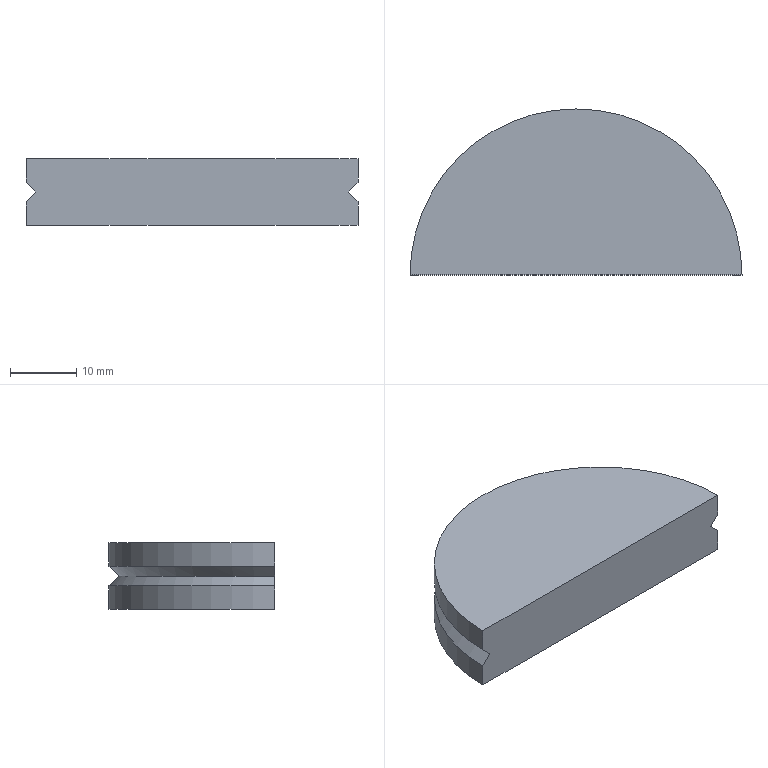Part | SolidWorks | features Extrusion 1, SweepCut 1 | 1 solid | 7 faces | box 50 x 25 x 10 mm | volume 9644 mm3 | plane 3 | cylinder 2 | cone 2 | commonest cylinder face diameters 50 x2
STEP:
#1=CARTESIAN_POINT('',(26.255,-21.468,10.));
#2=VERTEX_POINT('',#1);
#3=CARTESIAN_POINT('',(26.255,-21.468,6.5));
#4=VERTEX_POINT('',#3);
#5=CARTESIAN_POINT('',(26.255,-21.468,10.));
#6=DIRECTION('',(0.,0.,-1.));
#7=VECTOR('',#6,1000.);
#8=LINE('',#5,#7);
#9=EDGE_CURVE('',#2,#4,#8,.T.);
#10=ORIENTED_EDGE('',*,*,#9,.T.);
#11=CARTESIAN_POINT('',(-23.745,-21.468,6.5));
#12=VERTEX_POINT('',#11);
#13=CARTESIAN_POINT('',(1.255,-21.468,6.5));
#14=DIRECTION('',(0.,0.,-1.));
#15=DIRECTION('',(-1.,0.,0.));
#16=AXIS2_PLACEMENT_3D('',#13,#14,#15);
#17=CIRCLE('',#16,25.);
#18=EDGE_CURVE('',#12,#4,#17,.T.);
#19=ORIENTED_EDGE('',*,*,#18,.F.);
#20=CARTESIAN_POINT('',(-23.745,-21.468,10.));
#21=VERTEX_POINT('',#20);
#22=CARTESIAN_POINT('',(-23.745,-21.468,10.));
#23=DIRECTION('',(0.,0.,-1.));
#24=VECTOR('',#23,1000.);
#25=LINE('',#22,#24);
#26=EDGE_CURVE('',#21,#12,#25,.T.);
#27=ORIENTED_EDGE('',*,*,#26,.F.);
#28=CARTESIAN_POINT('',(1.255,-21.468,10.));
#29=DIRECTION('',(0.,0.,1.));
#30=DIRECTION('',(1.,0.,0.));
#31=AXIS2_PLACEMENT_3D('',#28,#29,#30);
#32=CIRCLE('',#31,25.);
#33=EDGE_CURVE('',#2,#21,#32,.T.);
#34=ORIENTED_EDGE('',*,*,#33,.F.);
#35=EDGE_LOOP('',(#10,#19,#27,#34));
#36=FACE_OUTER_BOUND('',#35,.T.);
#37=CARTESIAN_POINT('',(1.255,-21.468,10.));
#38=DIRECTION('',(0.,0.,-1.));
#39=DIRECTION('',(-1.,0.,0.));
#40=AXIS2_PLACEMENT_3D('',#37,#38,#39);
#41=CYLINDRICAL_SURFACE('',#40,25.);
#42=ADVANCED_FACE('',(#36),#41,.T.);
#43=CARTESIAN_POINT('',(-23.745,-21.468,3.5));
#44=VERTEX_POINT('',#43);
#45=CARTESIAN_POINT('',(-23.745,-21.468,0.));
#46=VERTEX_POINT('',#45);
#47=CARTESIAN_POINT('',(-23.745,-21.468,10.));
#48=DIRECTION('',(0.,0.,-1.));
#49=VECTOR('',#48,1000.);
#50=LINE('',#47,#49);
#51=EDGE_CURVE('',#44,#46,#50,.T.);
#52=ORIENTED_EDGE('',*,*,#51,.F.);
#53=CARTESIAN_POINT('',(26.255,-21.468,3.5));
#54=VERTEX_POINT('',#53);
#55=CARTESIAN_POINT('',(1.255,-21.468,3.5));
#56=DIRECTION('',(0.,0.,-1.));
#57=DIRECTION('',(-1.,0.,0.));
#58=AXIS2_PLACEMENT_3D('',#55,#56,#57);
#59=CIRCLE('',#58,25.);
#60=EDGE_CURVE('',#44,#54,#59,.T.);
#61=ORIENTED_EDGE('',*,*,#60,.T.);
#62=CARTESIAN_POINT('',(26.255,-21.468,0.));
#63=VERTEX_POINT('',#62);
#64=CARTESIAN_POINT('',(26.255,-21.468,10.));
#65=DIRECTION('',(0.,0.,-1.));
#66=VECTOR('',#65,1000.);
#67=LINE('',#64,#66);
#68=EDGE_CURVE('',#54,#63,#67,.T.);
#69=ORIENTED_EDGE('',*,*,#68,.T.);
#70=CARTESIAN_POINT('',(1.255,-21.468,0.));
#71=DIRECTION('',(0.,0.,1.));
#72=DIRECTION('',(1.,0.,0.));
#73=AXIS2_PLACEMENT_3D('',#70,#71,#72);
#74=CIRCLE('',#73,25.);
#75=EDGE_CURVE('',#63,#46,#74,.T.);
#76=ORIENTED_EDGE('',*,*,#75,.T.);
#77=EDGE_LOOP('',(#52,#61,#69,#76));
#78=FACE_OUTER_BOUND('',#77,.T.);
#79=CARTESIAN_POINT('',(1.255,-21.468,10.));
#80=DIRECTION('',(0.,0.,-1.));
#81=DIRECTION('',(-1.,0.,0.));
#82=AXIS2_PLACEMENT_3D('',#79,#80,#81);
#83=CYLINDRICAL_SURFACE('',#82,25.);
#84=ADVANCED_FACE('',(#78),#83,.T.);
#85=CARTESIAN_POINT('',(24.755,-21.468,5.));
#86=VERTEX_POINT('',#85);
#87=CARTESIAN_POINT('',(24.755,-21.468,5.));
#88=DIRECTION('',(0.7071,0.,-0.7071));
#89=VECTOR('',#88,1000.);
#90=LINE('',#87,#89);
#91=EDGE_CURVE('',#86,#54,#90,.T.);
#92=ORIENTED_EDGE('',*,*,#91,.F.);
#93=CARTESIAN_POINT('',(26.255,-21.468,6.5));
#94=DIRECTION('',(-0.7071,0.,-0.7071));
#95=VECTOR('',#94,1000.);
#96=LINE('',#93,#95);
#97=EDGE_CURVE('',#4,#86,#96,.T.);
#98=ORIENTED_EDGE('',*,*,#97,.F.);
#99=ORIENTED_EDGE('',*,*,#9,.F.);
#100=CARTESIAN_POINT('',(-23.745,-21.468,10.));
#101=DIRECTION('',(1.,0.,0.));
#102=VECTOR('',#101,1000.);
#103=LINE('',#100,#102);
#104=EDGE_CURVE('',#21,#2,#103,.T.);
#105=ORIENTED_EDGE('',*,*,#104,.F.);
#106=ORIENTED_EDGE('',*,*,#26,.T.);
#107=CARTESIAN_POINT('',(-22.245,-21.468,5.));
#108=VERTEX_POINT('',#107);
#109=CARTESIAN_POINT('',(-23.745,-21.468,6.5));
#110=DIRECTION('',(0.7071,0.,-0.7071));
#111=VECTOR('',#110,1000.);
#112=LINE('',#109,#111);
#113=EDGE_CURVE('',#12,#108,#112,.T.);
#114=ORIENTED_EDGE('',*,*,#113,.T.);
#115=CARTESIAN_POINT('',(-22.245,-21.468,5.));
#116=DIRECTION('',(-0.7071,0.,-0.7071));
#117=VECTOR('',#116,1000.);
#118=LINE('',#115,#117);
#119=EDGE_CURVE('',#108,#44,#118,.T.);
#120=ORIENTED_EDGE('',*,*,#119,.T.);
#121=ORIENTED_EDGE('',*,*,#51,.T.);
#122=CARTESIAN_POINT('',(-23.745,-21.468,0.));
#123=DIRECTION('',(1.,0.,0.));
#124=VECTOR('',#123,1000.);
#125=LINE('',#122,#124);
#126=EDGE_CURVE('',#46,#63,#125,.T.);
#127=ORIENTED_EDGE('',*,*,#126,.T.);
#128=ORIENTED_EDGE('',*,*,#68,.F.);
#129=EDGE_LOOP('',(#92,#98,#99,#105,#106,#114,#120,#121,#127,#128));
#130=FACE_OUTER_BOUND('',#129,.T.);
#131=CARTESIAN_POINT('',(-23.745,-21.468,10.));
#132=DIRECTION('',(0.,1.,0.));
#133=DIRECTION('',(0.,0.,1.));
#134=AXIS2_PLACEMENT_3D('',#131,#132,#133);
#135=PLANE('',#134);
#136=ADVANCED_FACE('',(#130),#135,.F.);
#137=ORIENTED_EDGE('',*,*,#33,.T.);
#138=ORIENTED_EDGE('',*,*,#104,.T.);
#139=EDGE_LOOP('',(#137,#138));
#140=FACE_OUTER_BOUND('',#139,.T.);
#141=CARTESIAN_POINT('',(1.255,-21.468,10.));
#142=DIRECTION('',(0.,0.,1.));
#143=DIRECTION('',(1.,0.,0.));
#144=AXIS2_PLACEMENT_3D('',#141,#142,#143);
#145=PLANE('',#144);
#146=ADVANCED_FACE('',(#140),#145,.T.);
#147=ORIENTED_EDGE('',*,*,#75,.F.);
#148=ORIENTED_EDGE('',*,*,#126,.F.);
#149=EDGE_LOOP('',(#147,#148));
#150=FACE_OUTER_BOUND('',#149,.T.);
#151=CARTESIAN_POINT('',(1.255,-21.468,0.));
#152=DIRECTION('',(0.,0.,1.));
#153=DIRECTION('',(1.,0.,0.));
#154=AXIS2_PLACEMENT_3D('',#151,#152,#153);
#155=PLANE('',#154);
#156=ADVANCED_FACE('',(#150),#155,.F.);
#157=CARTESIAN_POINT('',(1.255,-21.468,5.));
#158=DIRECTION('',(0.,0.,-1.));
#159=DIRECTION('',(-1.,0.,0.));
#160=AXIS2_PLACEMENT_3D('',#157,#158,#159);
#161=CIRCLE('',#160,23.5);
#162=EDGE_CURVE('',#108,#86,#161,.T.);
#163=ORIENTED_EDGE('',*,*,#162,.F.);
#164=ORIENTED_EDGE('',*,*,#113,.F.);
#165=ORIENTED_EDGE('',*,*,#18,.T.);
#166=ORIENTED_EDGE('',*,*,#97,.T.);
#167=EDGE_LOOP('',(#163,#164,#165,#166));
#168=FACE_OUTER_BOUND('',#167,.T.);
#169=CARTESIAN_POINT('',(1.255,-21.468,6.5));
#170=DIRECTION('',(0.,0.,1.));
#171=DIRECTION('',(1.,0.,0.));
#172=AXIS2_PLACEMENT_3D('',#169,#170,#171);
#173=CONICAL_SURFACE('',#172,25.,0.7854);
#174=ADVANCED_FACE('',(#168),#173,.T.);
#175=ORIENTED_EDGE('',*,*,#119,.F.);
#176=ORIENTED_EDGE('',*,*,#162,.T.);
#177=ORIENTED_EDGE('',*,*,#91,.T.);
#178=ORIENTED_EDGE('',*,*,#60,.F.);
#179=EDGE_LOOP('',(#175,#176,#177,#178));
#180=FACE_OUTER_BOUND('',#179,.T.);
#181=CARTESIAN_POINT('',(1.255,-21.468,5.));
#182=DIRECTION('',(0.,0.,-1.));
#183=DIRECTION('',(-1.,0.,0.));
#184=AXIS2_PLACEMENT_3D('',#181,#182,#183);
#185=CONICAL_SURFACE('',#184,23.5,0.7854);
#186=ADVANCED_FACE('',(#180),#185,.T.);
#187=CLOSED_SHELL('',(#42,#84,#136,#146,#156,#174,#186));
#188=MANIFOLD_SOLID_BREP('',#187);
#189=CARTESIAN_POINT('',(0.,0.,0.));
#190=DIRECTION('',(0.,0.,1.));
#191=DIRECTION('',(1.,0.,0.));
#192=AXIS2_PLACEMENT_3D('',#189,#190,#191);
#193=(LENGTH_UNIT()NAMED_UNIT(*)SI_UNIT(.MILLI.,.METRE.));
#194=UNCERTAINTY_MEASURE_WITH_UNIT(LENGTH_MEASURE(0.00001),#193,'','');
#195=(NAMED_UNIT(*)PLANE_ANGLE_UNIT()SI_UNIT($,.RADIAN.));
#196=(NAMED_UNIT(*)SI_UNIT($,.STERADIAN.)SOLID_ANGLE_UNIT());
#197=(GEOMETRIC_REPRESENTATION_CONTEXT(3)GLOBAL_UNCERTAINTY_ASSIGNED_CONTEXT((#194))GLOBAL_UNIT_ASSIGNED_CONTEXT((#193,#195,#196))REPRESENTATION_CONTEXT('',''));
#198=ADVANCED_BREP_SHAPE_REPRESENTATION('',(#188,#192),#197);